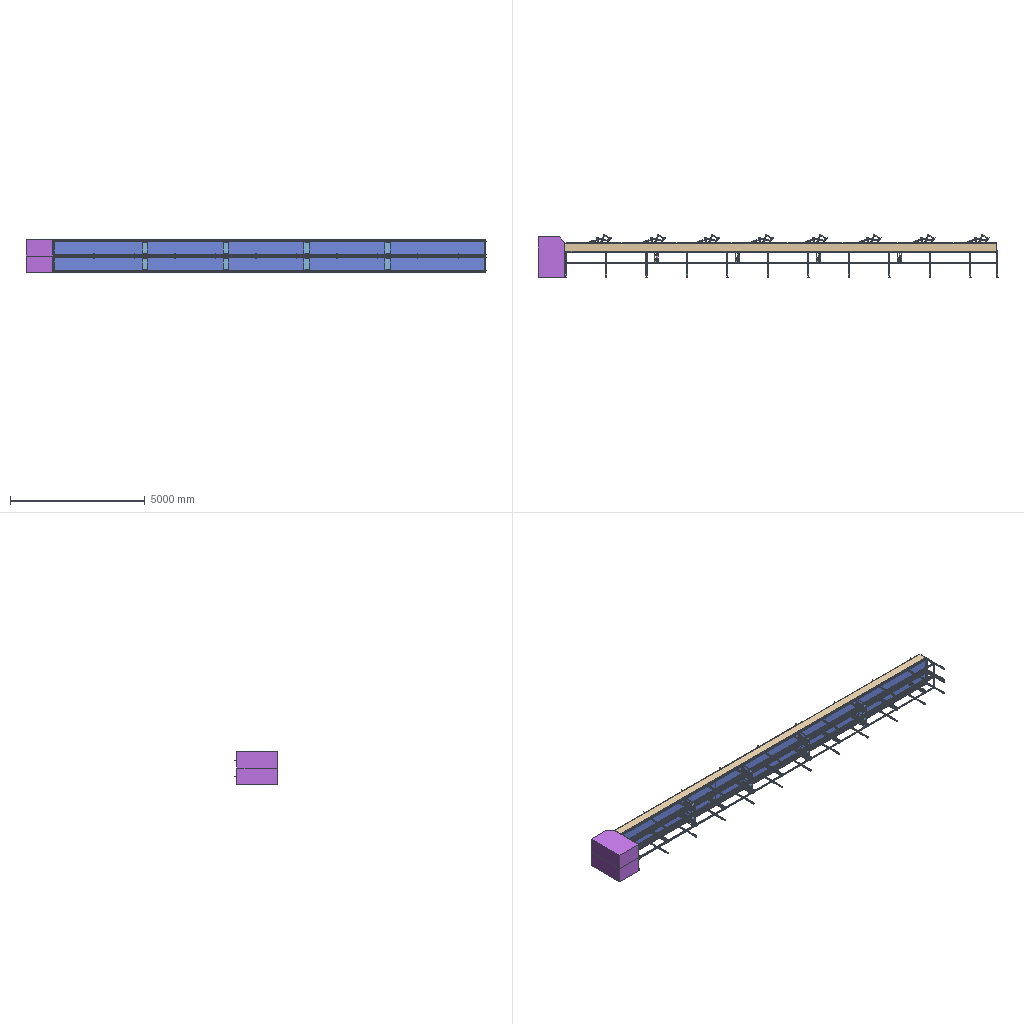Assembly | SolidWorks | 39 different items | 402 placed | box 17045 x 1585 x 1200 mm
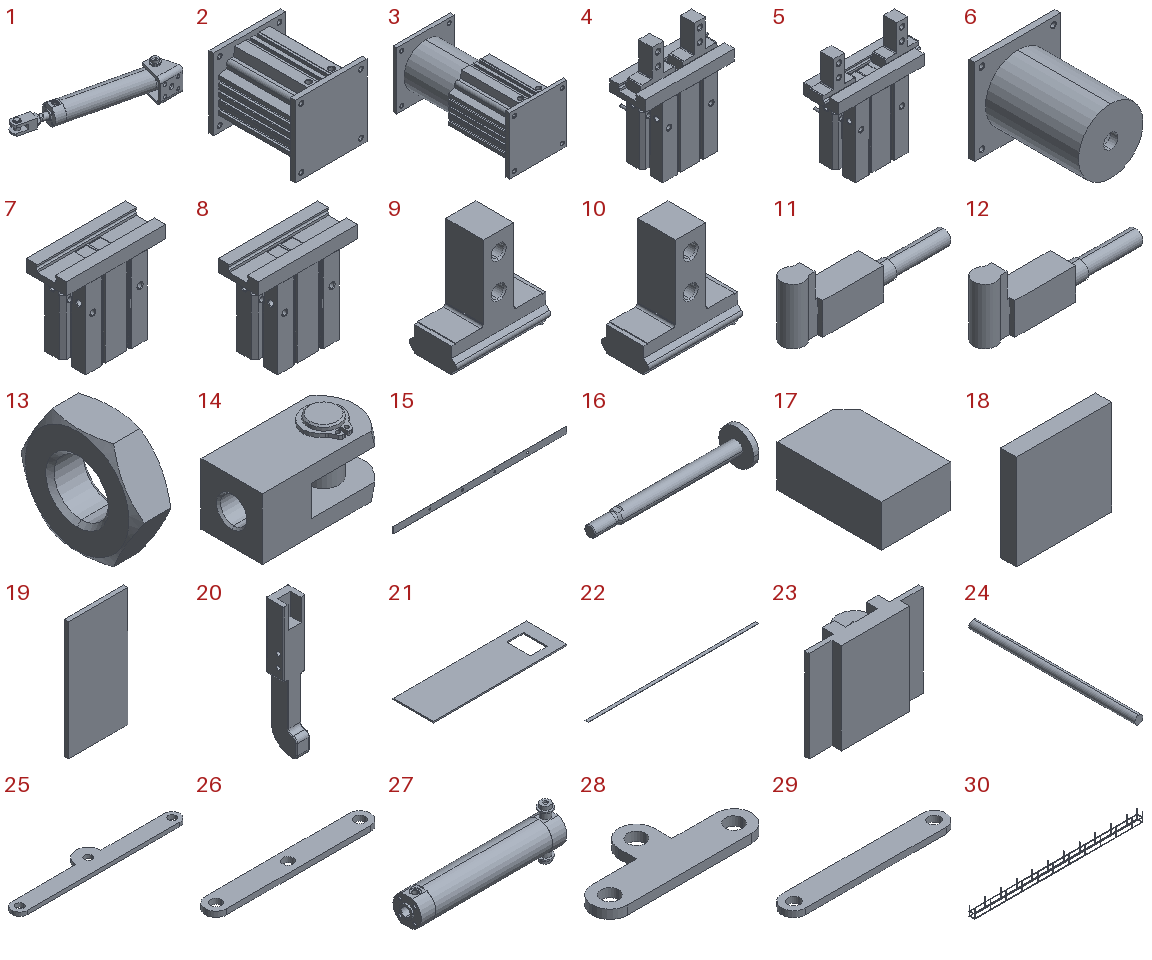Parts list (item | name | quantity | parent item | size | volume | features):
1 | (subassembly) | x16 | - | 272.662 x 101.563 x 67.7 mm | 211806 mm3 | features AEMSimFeature 1, CompositeCurve 1
2 | (subassembly) | x6 | - | 120 x 144.5 x 120 mm | 1424542 mm3 | features AEMSimFeature 1
3 | (subassembly) | x2 | - | 120 x 244.5 x 120 mm | 1424542 mm3 | features AEMSimFeature 1
4 | (subassembly) | x6 | - | 97 x 63.7 x 121.5 mm | 211309 mm3 | features AEMSimFeature 1, MirrorCompFeat 1, ReferencePattern 1
5 | (subassembly) | x2 | - | 109.088 x 63.7 x 121.5 mm | 211309 mm3 | features AEMSimFeature 1, MirrorCompFeat 1, ReferencePattern 1
6 | - | x2 | in 3 | 120 x 138 x 120 mm | 787135 mm3 | features BaseBody 1
7 | - | x6 | in 4 | 97 x 40 x 88 mm | 188244 mm3 | features BaseBody 1
8 | - | x2 | in 5 | 97 x 40 x 88 mm | 188244 mm3 | features BaseBody 1
9 | - | x12 | in 4 | 37.6 x 18.7 x 41.2 mm | 11010 mm3 | features BaseBody 1
10 | - | x4 | in 5 | 37.6 x 18.7 x 41.2 mm | 11010 mm3 | features BaseBody 1
11 | - | x12 | in 4 | 29 x 4.6 x 10 mm | 522.344 mm3 | features BaseBody 1
12 | - | x4 | in 5 | 29 x 4.6 x 10 mm | 522.344 mm3 | features BaseBody 1
13 | - | x16 | in 1 | 6 x 19.63 x 17 mm | 1117 mm3 | features BaseBody 1
14 | - | x16 | in 1 | 41 x 20 x 25.6 mm | 11481 mm3 | features BaseBody 1
15 | - | x2 | - | 16040 x 12 x 600 mm | 114266549 mm3 | features Cut 1, Extrusion 1, LPattern 1
16 | - | x16 | in 1 | 140 x 32 x 32 mm | 18387 mm3 | features BaseBody 1
17 | - | x2 | - | 1000 x 1500 x 600 mm | 888000000 mm3 | features Chamfer 1, Extrusion 1
18 | - | x8 | - | 120 x 20 x 120 mm | 288000 mm3 | features Extrusion 1
19 | - | x8 | - | 200 x 15 x 400 mm | 1194970 mm3 | features Extrusion 1, HoleWzd 1
20 | - | x16 | - | 25 x 30 x 150 mm | 55771 mm3 | features Fillet 5, ICE 3, Cut 1, Extrusion 1, HoleWzd 1
21 | - | x16 | - | 2000 x 600 x 71 mm | 22419827 mm3 | features ICE 3, Cut 1, Extrusion 1, Fillet 1, LPattern 1
22 | - | x4 | - | 16000 x 300 x 20 mm | 96000000 mm3 | features Extrusion 1
23 | - | x2 | - | 500 x 165 x 400 mm | 11247754 mm3 | features ICE 4, Extrusion 1
24 | - | x32 | - | 20 x 400 x 20 mm | 125664 mm3 | features Extrusion 1
25 | - | x16 | - | 440 x 72.879 x 10 mm | 180122 mm3 | features ICE 3, Extrusion 1
26 | - | x16 | - | 310 x 40 x 10 mm | 111142 mm3 | features ICE 2, Extrusion 1
27 | - | x16 | in 1 | 201 x 38.4 x 67.7 mm | 158139 mm3 | features BaseBody 1
28 | - | x16 | - | 180 x 80 x 10 mm | 73425 mm3 | features ICE 3, Extrusion 1, Fillet 1
29 | - | x16 | - | 275 x 40 x 10 mm | 100283 mm3 | features Extrusion 1, ICE 1
30 | - | x2 | - | - | 48717671 mm3 | features LPattern 2, 3DProfileFeature 1, WeldMemberFeat 1, WeldmentFeature 1
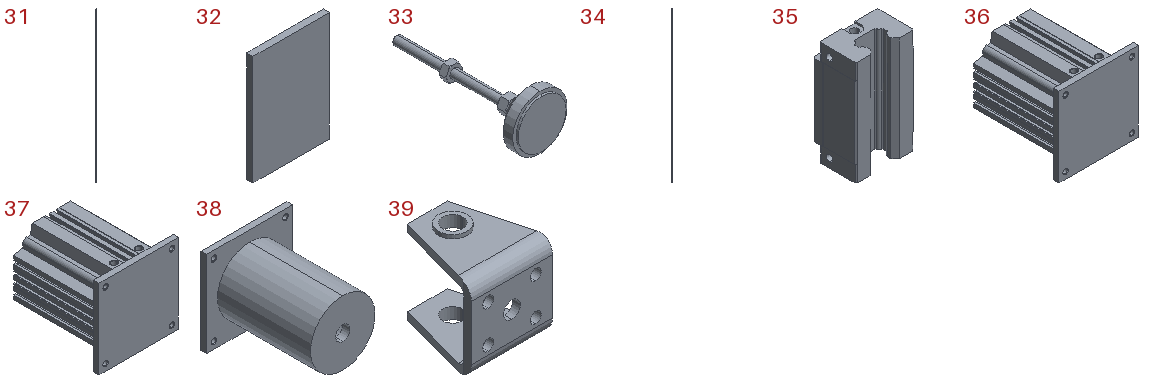31 | - | x2 | - | 30 x 30 x 5500 mm | 3887721 mm3 | features Extrusion 1
32 | - | x16 | - | 250 x 70 x 360 mm | 1902431 mm3 | features Cut 1, Extrusion 1, Fillet 1, ICE 1
33 | - | x48 | - | 50 x 134.1 x 50 mm | 39920 mm3 | features BaseBody 2
34 | - | x4 | - | 23 x 22 x 16040 mm | 6693240 mm3 | features ICE 3, BaseBody 1, LPattern 1
35 | - | x8 | - | 48 x 34.5 x 84 mm | 100839 mm3 | features BaseBody 1
36 | - | x6 | in 2 | 120 x 136.5 x 120 mm | 637407 mm3 | features BaseBody 1
37 | - | x2 | in 3 | 120 x 136.5 x 120 mm | 637407 mm3 | features BaseBody 1
38 | - | x6 | in 2 | 120 x 138 x 120 mm | 787135 mm3 | features BaseBody 1
39 | - | x16 | in 1 | 48 x 50 x 53.8 mm | 22684 mm3 | features BaseBody 1
Mates (type | each side: item.copy, entity, surface, feature):
In the top assembly
Coincident | 30.1 plane | assembly plane | 3 times
Width | 17.1 face plane Boss-Extrude1 | 17.1 face plane Boss-Extrude1 | 30.1 face plane Aohong aluminium profile 001.08.40.40(1) | 30.1 face plane Aohong aluminium profile 001.08.40.40(1)
Coincident | 30.1 face plane Aohong aluminium profile 001.08.40.40(1) | 17.1 face plane Boss-Extrude1
Concentric | 30.1 face cylinder Aohong aluminium profile 001.08.40.40(1) | 33.1 face cylinder Base body^1753149266374_DABJ-50~DABJ-80-1-solid1
Coincident | 30.1 face plane Aohong aluminium profile 001.08.40.40(1) | 33.1 face plane Base body^1753149266374_DABJ-50-1-solid1
Concentric | 30.1 face cylinder Aohong aluminium profile 001.08.40.40(1) | 33.2 face cylinder Base body^1753149266374_DABJ-50~DABJ-80-1-solid1
Coincident | 33.1 face plane Base body^1753149266374_DABJ-50~DABJ-80-1-solid1 | 33.2 face plane Base body^1753149266374_DABJ-50~DABJ-80-1-solid1
Concentric | 30.1 face cylinder Aohong aluminium profile 001.08.40.40(1) | 33.3 face cylinder Base body^1753149266374_DABJ-50~DABJ-80-1-solid1
Coincident | 30.1 face plane Aohong aluminium profile 001.08.40.40(1) | 33.3 face plane Base body^1753149266374_DABJ-50-1-solid1
Concentric | 30.1 face cylinder Aohong aluminium profile 001.08.40.40(1) | 33.4 face cylinder Base body^1753149266374_DABJ-50~DABJ-80-1-solid1
Coincident | 33.3 face plane Base body^1753149266374_DABJ-50~DABJ-80-1-solid1 | 33.4 face plane Base body^1753149266374_DABJ-50~DABJ-80-1-solid1
Coincident | 17.1 face plane Boss-Extrude1 | 33.1 face plane Base body^1753149266374_DABJ-50~DABJ-80-1-solid1
Coincident | 30.1 face plane Aohong aluminium profile 001.08.40.40(1) | 15.1 face plane Boss-Extrude1
Coincident | 17.1 face plane Boss-Extrude1 | 15.1 face plane Boss-Extrude1
Width | 15.1 face plane Boss-Extrude1 | 15.1 face plane Boss-Extrude1 | 30.1 face plane Aohong aluminium profile 001.08.40.40(1) | 30.1 face plane Aohong aluminium profile 001.08.40.40(1)
Coincident | 15.1 face plane Boss-Extrude1 | 34.1 face plane Input3
Parallel | 15.1 face plane Boss-Extrude1 | 34.1 face plane Input3
Coincident | 17.1 face plane Boss-Extrude1 | 34.1 face plane Input3
Coincident | 35.1 face plane Input1 | 34.1 face plane Input3
Width | 34.1 face plane Input3 | 34.1 face plane Input3 | 35.1 face plane Input1 | 35.1 face plane Input1
Coincident | 35.1 face plane Input1 | 35.2 face plane Input1 | 2 times
DistanceDim | 35.1 face plane Input1 | 35.2 face plane Input1
Width | 34.1 face plane Input3 | 34.2 face plane Input3 | 15.1 face plane Boss-Extrude1 | 15.1 face plane Boss-Extrude1
Coincident | 35.1 face plane Input1 | 23.1 face plane Boss-Extrude1
Width | 23.1 face plane Boss-Extrude1 | 23.1 face plane Boss-Extrude1 | 15.1 face plane Boss-Extrude1 | 15.1 face plane Boss-Extrude1
Width | 23.1 face plane Boss-Extrude1 | 23.1 face plane Boss-Extrude1 | 35.1 face plane Input1 | 35.2 face plane Input1
Coincident | 15.1 face plane Boss-Extrude1 | 22.1 face plane Boss-Extrude1 | 2 times
Coincident | 17.1 face plane Boss-Extrude1 | 22.1 face plane Boss-Extrude1
Coincident | 15.1 face plane Boss-Extrude1 | 22.2 face plane Boss-Extrude1
Coincident | 22.1 face plane Boss-Extrude1 | 22.2 face plane Boss-Extrude1
Coincident | 17.1 face plane Boss-Extrude1 | 22.2 face plane Boss-Extrude1
Coincident | 17.1 face plane Boss-Extrude1 | 21.1 face plane Boss-Extrude1
Coincident | 22.2 face plane Boss-Extrude1 | 21.1 face plane Boss-Extrude1 | 2 times
Coincident | 21.1 face plane Cut-Extrude1 | 32.1 face plane Boss-Extrude1
Coincident | 21.1 edge | 32.1 edge
Coincident | 15.1 face plane Boss-Extrude1 | 24.1 face plane Boss-Extrude1
Concentric | 24.1 face cylinder Boss-Extrude1 | 19.1 edge
Coincident | 24.1 face plane Boss-Extrude1 | 19.1 edge
Width | 19.1 face plane Boss-Extrude1 | 19.1 face plane Boss-Extrude1 | 30.1 face plane Aohong aluminium profile 001.08.40.40(1) | 30.1 face plane Aohong aluminium profile 001.08.40.40(1)
Coincident | 19.1 face plane Boss-Extrude1 | 37.1 face plane MGF40-100(0)_BODY(1)
Width | 37.1 face plane MGF40-100(0)_BODY(1) | 37.1 face plane MGF40-100(0)_BODY(1) | 19.1 face plane Boss-Extrude1 | 19.1 face plane Boss-Extrude1 | 2 times
Coincident | 6.1 edge | 18.1 face plane Boss-Extrude1 | 2 times
Coincident | 6.1 face plane MGF40-100(0)_TABLE(1) | 18.1 face plane Boss-Extrude1 | 3 times
Concentric | 32.1 face cylinder Cut-Extrude1 | 29.1 face cylinder Cut-Extrude1
Coincident | 32.1 face plane Boss-Extrude2 | 29.1 face plane Boss-Extrude1
Concentric | 32.1 edge | 25.1 edge
Coincident | 29.1 face plane Boss-Extrude1 | 25.1 face plane Boss-Extrude1
Concentric | 29.1 edge | 26.1 edge
Coincident | 29.1 face plane Boss-Extrude1 | 26.1 face plane Boss-Extrude1
Concentric | 21.1 face cylinder Cut-Extrude3 | 26.1 edge
Concentric | 25.1 edge | 28.1 edge
Coincident | 25.1 face plane Boss-Extrude1 | 28.1 face plane Boss-Extrude1
Concentric | 21.1 edge | 28.1 edge
Coincident | 21.1 face plane Boss-Extrude1 | 39.1 face plane CG-032-24A(1)
Coincident | 28.1 face plane Boss-Extrude1 | 14.1 face plane Y-G03_CG1-Z(1)
Concentric | 28.1 face cylinder Cut-Extrude2 | 14.1 face cylinder Y-G03_CG1-Z(1)
Concentric | 23.1 face cylinder Cut-Extrude2 | 31.1 face cylinder Boss-Extrude1
Coincident | 19.2 face plane Boss-Extrude1 | 36.1 face plane MGF40-100(0)_BODY(1)
Coincident | 37.1 face plane MGF40-100(0)_BODY(1) | 36.1 face plane MGF40-100(0)_BODY(1)
Width | 36.1 face plane MGF40-100(0)_BODY(1) | 36.1 face plane MGF40-100(0)_BODY(1) | 19.2 face plane Boss-Extrude1 | 19.2 face plane Boss-Extrude1
Coincident | 38.1 face plane MGF40-100(0)_TABLE(1) | 18.2 face plane Boss-Extrude1 | 3 times
Coincident | 18.1 face plane Boss-Extrude1 | 8.1 face plane MHZ2-32C1_Body(1)
Width | 8.1 face plane MHZ2-32C1_Body(1) | 8.1 face plane MHZ2-32C1_Body(1) | 18.1 face plane Boss-Extrude1 | 18.1 face plane Boss-Extrude1
Width | 18.1 face plane Boss-Extrude1 | 18.1 face plane Boss-Extrude1 | 8.1 face plane MHZ2-32C1_Body(1) | 8.1 face plane MHZ2-32C1_Body(1)
Coincident | 10.1 face plane MHZ2-32C1_Finger(1) | 20.1 face plane Cut-Extrude1 | 3 times
Parallel | 10.1 face plane MHZ2-32C1_Finger(1) | 20.1 face plane Boss-Extrude1
Coincident | 20.1 face plane Boss-Extrude1 | 20.2 face plane Boss-Extrude1 | 2 times
Coincident | 10.2 face plane MHZ2-32C1_Finger(1) | 20.2 face plane Cut-Extrude1
DistanceDim | 19.1 face plane Boss-Extrude1 | 17.1 face plane Boss-Extrude1
Coincident | 18.2 face plane Boss-Extrude1 | 7.1 face plane MHZ2-32C1_Body(1)
Coincident | 8.1 face plane MHZ2-32C1_Body(1) | 7.1 face plane MHZ2-32C1_Body(1)
Width | 7.1 face plane MHZ2-32C1_Body(1) | 7.1 face plane MHZ2-32C1_Body(1) | 18.2 face plane Boss-Extrude1 | 18.2 face plane Boss-Extrude1
Coincident | 9.1 face plane MHZ2-32C1_Finger(1) | 20.3 face plane Cut-Extrude1 | 3 times
Coincident | 20.3 face plane Boss-Extrude1 | 20.4 face plane Boss-Extrude1 | 2 times
Coincident | 9.2 face plane MHZ2-32C1_Finger(1) | 20.4 face plane Cut-Extrude1
In subassembly 4
Width | 9.3 face plane MHZ2-32C1_Finger(1) | 9.3 face plane MHZ2-32C1_Finger(1) | 7.2 face plane MHZ2-32C1_Body(1) | 7.2 face plane MHZ2-32C1_Body(1)
Coincident | 7.2 face plane MHZ2-32C1_Body(1) | 9.3 face plane MHZ2-32C1_Finger(1)
In subassembly 2
Concentric | 36.2 face cylinder MGF40-100(0)_BODY(1) | 38.2 face cylinder MGF40-100(0)_TABLE(1)
Parallel | 36.2 face plane MGF40-100(0)_BODY(1) | 38.2 face plane MGF40-100(0)_TABLE(1)
LimitDistanceDim | 36.2 face plane MGF40-100(0)_BODY(1) | 38.2 face plane MGF40-100(0)_TABLE(1)
In subassembly 1
Concentric | 27.1 face cylinder CG1TN32-76SZ1(0)_BODY(1) | 39.2 face cylinder CG-032-24A(1)
Coincident | 27.1 face plane CG1TN32-76SZ1(0)_BODY(1) | 39.2 face plane CG-032-24A(1)
Concentric | 27.1 face cylinder CG1TN32-76SZ1(0)_BODY(1) | 16.1 face cylinder CG132-76Z1_ST(0)_ROD(1)
Concentric | 16.1 face cylinder CG132-76Z1_ST(0)_ROD(1) | 13.1 face cylinder NT-03-25A-CG1(1)
Concentric | 16.1 face cylinder CG132-76Z1_ST(0)_ROD(1) | 14.2 face cylinder Y-G03_CG1-Z(1)
Coincident | 13.1 face plane NT-03-25A-CG1(1) | 14.2 face plane Y-G03_CG1-Z(1)
Coincident | 16.1 edge | 13.1 face plane NT-03-25A-CG1(1)
Parallel | 27.1 face plane CG1TN32-76SZ1(0)_BODY(1) | 14.2 face plane Y-G03_CG1-Z(1)
LimitDistanceDim | 27.1 face plane CG1TN32-76SZ1(0)_BODY(1) | 16.1 face plane CG132-76Z1_ST(0)_ROD(1)
In subassembly 3
Concentric | 37.2 face cylinder MGF40-100(0)_BODY(1) | 6.2 face cylinder MGF40-100(0)_TABLE(1)
Parallel | 37.2 face plane MGF40-100(0)_BODY(1) | 6.2 face plane MGF40-100(0)_TABLE(1)
LimitDistanceDim | 37.2 face plane MGF40-100(0)_BODY(1) | 6.2 face plane MGF40-100(0)_TABLE(1)
In subassembly 5
Width | 10.3 face plane MHZ2-32C1_Finger(1) | 10.3 face plane MHZ2-32C1_Finger(1) | 8.2 face plane MHZ2-32C1_Body(1) | 8.2 face plane MHZ2-32C1_Body(1)
Coincident | 8.2 face plane MHZ2-32C1_Body(1) | 10.3 face plane MHZ2-32C1_Finger(1)